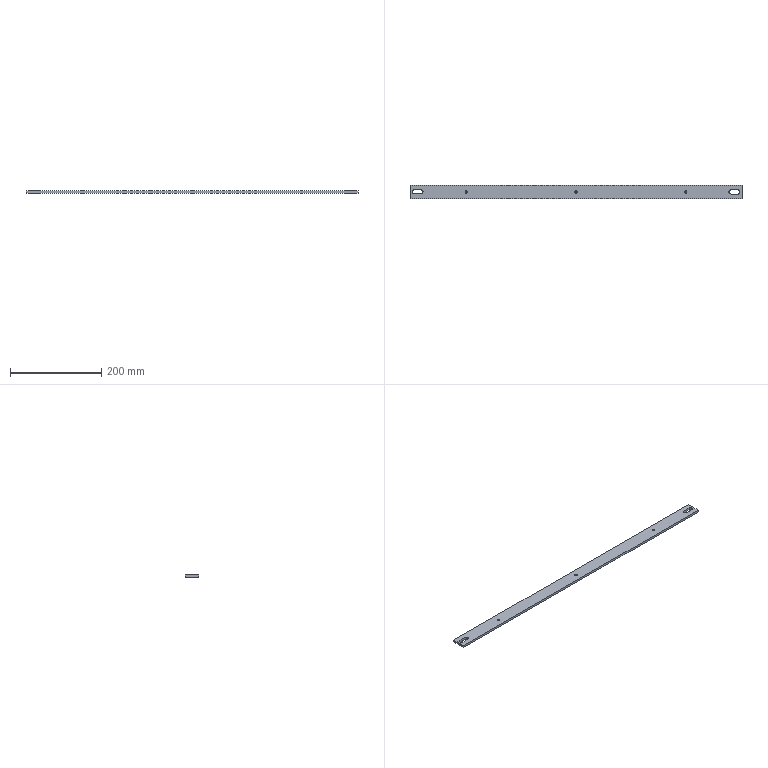Part | STEP file | 1 solid | 22 faces | box 726 x 30 x 5 mm | volume 106619 mm3 | cylinder 12 | plane 10 | commonest cylinder face diameters 5 x6 9 x6